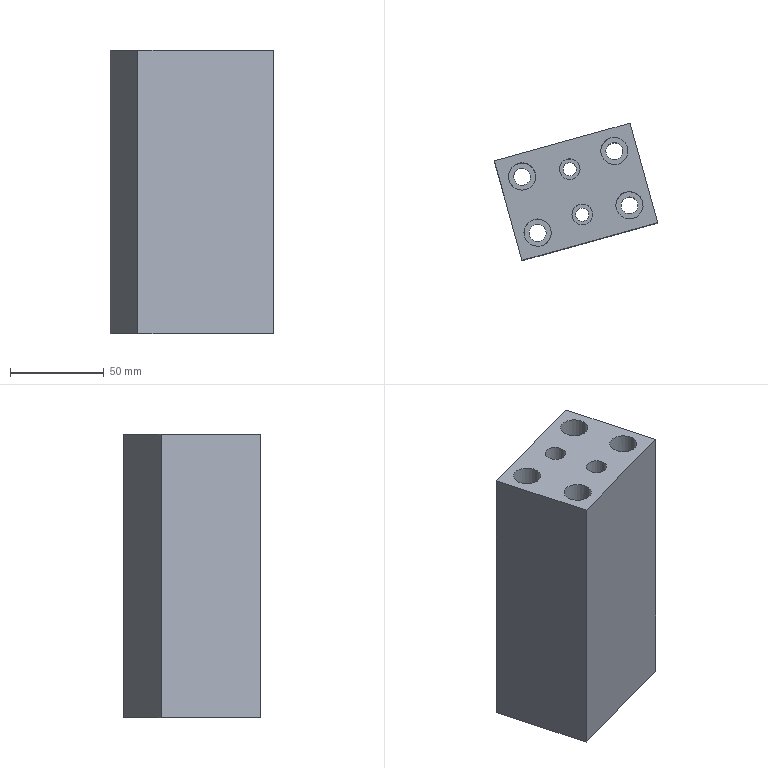Part | NX | features solid 2 | 1 solid | 26 faces | box 86.97 x 73.043 x 151.131 mm | volume 455545 mm3 | plane 13 | cylinder 13 | commonest cylinder face diameters 9.007 x4 14.508 x4 7 x2 11 x2 41 x1
STEP:
#1=CARTESIAN_POINT('',(1601.628,0.6566,173.999));
#2=VERTEX_POINT('',#1);
#3=CARTESIAN_POINT('',(1602.832,-3.683,173.999));
#4=DIRECTION('',(0.,0.,-1.));
#5=DIRECTION('',(-0.2672,0.9636,0.));
#6=AXIS2_PLACEMENT_3D('',#3,#4,#5);
#7=CIRCLE('',#6,4.503);
#8=EDGE_CURVE('',#2,#2,#7,.T.);
#9=ORIENTED_EDGE('',*,*,#8,.T.);
#10=EDGE_LOOP('',(#9));
#11=FACE_BOUND('',#10,.T.);
#12=CARTESIAN_POINT('',(1600.893,3.307,173.999));
#13=VERTEX_POINT('',#12);
#14=CARTESIAN_POINT('',(1602.832,-3.683,173.999));
#15=DIRECTION('',(0.,0.,1.));
#16=DIRECTION('',(-0.2672,0.9636,0.));
#17=AXIS2_PLACEMENT_3D('',#14,#15,#16);
#18=CIRCLE('',#17,7.254);
#19=EDGE_CURVE('',#13,#13,#18,.F.);
#20=ORIENTED_EDGE('',*,*,#19,.F.);
#21=EDGE_LOOP('',(#20));
#22=FACE_BOUND('',#21,.T.);
#23=CARTESIAN_POINT('',(1602.832,-3.683,173.999));
#24=DIRECTION('',(0.,0.,-1.));
#25=DIRECTION('',(-0.2672,0.9636,0.));
#26=AXIS2_PLACEMENT_3D('',#23,#24,#25);
#27=PLANE('',#26);
#28=ADVANCED_FACE('',(#11,#22),#27,.F.);
#29=ORIENTED_EDGE('',*,*,#8,.F.);
#30=EDGE_LOOP('',(#29));
#31=FACE_BOUND('',#30,.T.);
#32=CARTESIAN_POINT('',(1601.628,0.6566,94.999));
#33=VERTEX_POINT('',#32);
#34=CARTESIAN_POINT('',(1602.832,-3.683,94.999));
#35=DIRECTION('',(0.,0.,-1.));
#36=DIRECTION('',(-0.2672,0.9636,0.));
#37=AXIS2_PLACEMENT_3D('',#34,#35,#36);
#38=CIRCLE('',#37,4.503);
#39=EDGE_CURVE('',#33,#33,#38,.T.);
#40=ORIENTED_EDGE('',*,*,#39,.T.);
#41=EDGE_LOOP('',(#40));
#42=FACE_BOUND('',#41,.T.);
#43=CARTESIAN_POINT('',(1602.832,-3.683,187.999));
#44=DIRECTION('',(0.,0.,-1.));
#45=DIRECTION('',(-0.2672,0.9636,0.));
#46=AXIS2_PLACEMENT_3D('',#43,#44,#45);
#47=CYLINDRICAL_SURFACE('',#46,4.503);
#48=ADVANCED_FACE('',(#31,#42),#47,.F.);
#49=ORIENTED_EDGE('',*,*,#19,.T.);
#50=EDGE_LOOP('',(#49));
#51=FACE_BOUND('',#50,.T.);
#52=CARTESIAN_POINT('',(1595.578,-3.683,246.13));
#53=VERTEX_POINT('',#52);
#54=CARTESIAN_POINT('',(1602.832,-3.683,246.13));
#55=DIRECTION('',(0.,0.,-1.));
#56=DIRECTION('',(-1.,0.,0.));
#57=AXIS2_PLACEMENT_3D('',#54,#55,#56);
#58=CIRCLE('',#57,7.254);
#59=EDGE_CURVE('',#53,#53,#58,.F.);
#60=ORIENTED_EDGE('',*,*,#59,.T.);
#61=EDGE_LOOP('',(#60));
#62=FACE_BOUND('',#61,.T.);
#63=CARTESIAN_POINT('',(1602.832,-3.683,184.999));
#64=DIRECTION('',(0.,0.,-1.));
#65=DIRECTION('',(-0.2672,0.9636,0.));
#66=AXIS2_PLACEMENT_3D('',#63,#64,#65);
#67=CYLINDRICAL_SURFACE('',#66,7.254);
#68=ADVANCED_FACE('',(#51,#62),#67,.F.);
#69=CARTESIAN_POINT('',(1616.422,30.113,159.999));
#70=VERTEX_POINT('',#69);
#71=CARTESIAN_POINT('',(1619.922,30.113,159.999));
#72=DIRECTION('',(0.,0.,-1.));
#73=DIRECTION('',(-1.,0.,0.));
#74=AXIS2_PLACEMENT_3D('',#71,#72,#73);
#75=CIRCLE('',#74,3.5);
#76=EDGE_CURVE('',#70,#70,#75,.F.);
#77=ORIENTED_EDGE('',*,*,#76,.F.);
#78=EDGE_LOOP('',(#77));
#79=FACE_BOUND('',#78,.T.);
#80=CARTESIAN_POINT('',(1616.422,30.113,178.999));
#81=VERTEX_POINT('',#80);
#82=CARTESIAN_POINT('',(1619.922,30.113,178.999));
#83=DIRECTION('',(0.,0.,-1.));
#84=DIRECTION('',(-1.,0.,0.));
#85=AXIS2_PLACEMENT_3D('',#82,#83,#84);
#86=CIRCLE('',#85,3.5);
#87=EDGE_CURVE('',#81,#81,#86,.T.);
#88=ORIENTED_EDGE('',*,*,#87,.F.);
#89=EDGE_LOOP('',(#88));
#90=FACE_BOUND('',#89,.T.);
#91=CARTESIAN_POINT('',(1619.922,30.113,201.999));
#92=DIRECTION('',(0.,0.,-1.));
#93=DIRECTION('',(0.2672,-0.9636,0.));
#94=AXIS2_PLACEMENT_3D('',#91,#92,#93);
#95=CYLINDRICAL_SURFACE('',#94,3.5);
#96=ADVANCED_FACE('',(#79,#90),#95,.F.);
#97=CARTESIAN_POINT('',(1623.102,6.022,159.999));
#98=VERTEX_POINT('',#97);
#99=CARTESIAN_POINT('',(1626.602,6.022,159.999));
#100=DIRECTION('',(0.,0.,-1.));
#101=DIRECTION('',(-1.,0.,0.));
#102=AXIS2_PLACEMENT_3D('',#99,#100,#101);
#103=CIRCLE('',#102,3.5);
#104=EDGE_CURVE('',#98,#98,#103,.F.);
#105=ORIENTED_EDGE('',*,*,#104,.F.);
#106=EDGE_LOOP('',(#105));
#107=FACE_BOUND('',#106,.T.);
#108=CARTESIAN_POINT('',(1623.102,6.022,178.999));
#109=VERTEX_POINT('',#108);
#110=CARTESIAN_POINT('',(1626.602,6.022,178.999));
#111=DIRECTION('',(0.,0.,-1.));
#112=DIRECTION('',(-1.,0.,0.));
#113=AXIS2_PLACEMENT_3D('',#110,#111,#112);
#114=CIRCLE('',#113,3.5);
#115=EDGE_CURVE('',#109,#109,#114,.T.);
#116=ORIENTED_EDGE('',*,*,#115,.F.);
#117=EDGE_LOOP('',(#116));
#118=FACE_BOUND('',#117,.T.);
#119=CARTESIAN_POINT('',(1626.602,6.022,201.999));
#120=DIRECTION('',(0.,0.,-1.));
#121=DIRECTION('',(0.2672,-0.9636,0.));
#122=AXIS2_PLACEMENT_3D('',#119,#120,#121);
#123=CYLINDRICAL_SURFACE('',#122,3.5);
#124=ADVANCED_FACE('',(#107,#118),#123,.F.);
#125=ORIENTED_EDGE('',*,*,#115,.T.);
#126=EDGE_LOOP('',(#125));
#127=FACE_BOUND('',#126,.T.);
#128=CARTESIAN_POINT('',(1621.102,6.022,178.999));
#129=VERTEX_POINT('',#128);
#130=CARTESIAN_POINT('',(1626.602,6.022,178.999));
#131=DIRECTION('',(0.,0.,-1.));
#132=DIRECTION('',(-1.,0.,0.));
#133=AXIS2_PLACEMENT_3D('',#130,#131,#132);
#134=CIRCLE('',#133,5.5);
#135=EDGE_CURVE('',#129,#129,#134,.T.);
#136=ORIENTED_EDGE('',*,*,#135,.F.);
#137=EDGE_LOOP('',(#136));
#138=FACE_BOUND('',#137,.T.);
#139=CARTESIAN_POINT('',(1626.602,6.022,178.999));
#140=DIRECTION('',(0.,0.,-1.));
#141=DIRECTION('',(-0.2672,0.9636,0.));
#142=AXIS2_PLACEMENT_3D('',#139,#140,#141);
#143=PLANE('',#142);
#144=ADVANCED_FACE('',(#127,#138),#143,.F.);
#145=ORIENTED_EDGE('',*,*,#87,.T.);
#146=EDGE_LOOP('',(#145));
#147=FACE_BOUND('',#146,.T.);
#148=CARTESIAN_POINT('',(1614.422,30.113,178.999));
#149=VERTEX_POINT('',#148);
#150=CARTESIAN_POINT('',(1619.922,30.113,178.999));
#151=DIRECTION('',(0.,0.,-1.));
#152=DIRECTION('',(-1.,0.,0.));
#153=AXIS2_PLACEMENT_3D('',#150,#151,#152);
#154=CIRCLE('',#153,5.5);
#155=EDGE_CURVE('',#149,#149,#154,.T.);
#156=ORIENTED_EDGE('',*,*,#155,.F.);
#157=EDGE_LOOP('',(#156));
#158=FACE_BOUND('',#157,.T.);
#159=CARTESIAN_POINT('',(1619.922,30.113,178.999));
#160=DIRECTION('',(0.,0.,-1.));
#161=DIRECTION('',(-0.2672,0.9636,0.));
#162=AXIS2_PLACEMENT_3D('',#159,#160,#161);
#163=PLANE('',#162);
#164=ADVANCED_FACE('',(#147,#158),#163,.F.);
#165=ORIENTED_EDGE('',*,*,#104,.T.);
#166=EDGE_LOOP('',(#165));
#167=FACE_BOUND('',#166,.T.);
#168=CARTESIAN_POINT('',(1617.784,37.822,159.999));
#169=VERTEX_POINT('',#168);
#170=CARTESIAN_POINT('',(1623.262,18.068,159.999));
#171=DIRECTION('',(0.,0.,-1.));
#172=DIRECTION('',(-0.2672,0.9636,0.));
#173=AXIS2_PLACEMENT_3D('',#170,#171,#172);
#174=CIRCLE('',#173,20.5);
#175=EDGE_CURVE('',#169,#169,#174,.T.);
#176=ORIENTED_EDGE('',*,*,#175,.T.);
#177=EDGE_LOOP('',(#176));
#178=FACE_BOUND('',#177,.T.);
#179=ORIENTED_EDGE('',*,*,#76,.T.);
#180=EDGE_LOOP('',(#179));
#181=FACE_BOUND('',#180,.T.);
#182=CARTESIAN_POINT('',(1623.262,18.068,159.999));
#183=DIRECTION('',(0.,0.,-1.));
#184=DIRECTION('',(-0.2672,0.9636,0.));
#185=AXIS2_PLACEMENT_3D('',#182,#183,#184);
#186=PLANE('',#185);
#187=ADVANCED_FACE('',(#167,#178,#181),#186,.T.);
#188=CARTESIAN_POINT('',(1652.913,6.57,173.999));
#189=VERTEX_POINT('',#188);
#190=CARTESIAN_POINT('',(1651.71,10.91,173.999));
#191=DIRECTION('',(0.,0.,1.));
#192=DIRECTION('',(0.2672,-0.9636,0.));
#193=AXIS2_PLACEMENT_3D('',#190,#191,#192);
#194=CIRCLE('',#193,4.503);
#195=EDGE_CURVE('',#189,#189,#194,.F.);
#196=ORIENTED_EDGE('',*,*,#195,.T.);
#197=EDGE_LOOP('',(#196));
#198=FACE_BOUND('',#197,.T.);
#199=CARTESIAN_POINT('',(1653.648,3.92,173.999));
#200=VERTEX_POINT('',#199);
#201=CARTESIAN_POINT('',(1651.71,10.91,173.999));
#202=DIRECTION('',(0.,0.,-1.));
#203=DIRECTION('',(0.2672,-0.9636,0.));
#204=AXIS2_PLACEMENT_3D('',#201,#202,#203);
#205=CIRCLE('',#204,7.254);
#206=EDGE_CURVE('',#200,#200,#205,.T.);
#207=ORIENTED_EDGE('',*,*,#206,.F.);
#208=EDGE_LOOP('',(#207));
#209=FACE_BOUND('',#208,.T.);
#210=CARTESIAN_POINT('',(1651.71,10.91,173.999));
#211=DIRECTION('',(0.,0.,-1.));
#212=DIRECTION('',(0.2672,-0.9636,0.));
#213=AXIS2_PLACEMENT_3D('',#210,#211,#212);
#214=PLANE('',#213);
#215=ADVANCED_FACE('',(#198,#209),#214,.F.);
#216=CARTESIAN_POINT('',(1644.896,35.479,173.999));
#217=VERTEX_POINT('',#216);
#218=CARTESIAN_POINT('',(1643.692,39.819,173.999));
#219=DIRECTION('',(0.,0.,1.));
#220=DIRECTION('',(0.2672,-0.9636,0.));
#221=AXIS2_PLACEMENT_3D('',#218,#219,#220);
#222=CIRCLE('',#221,4.503);
#223=EDGE_CURVE('',#217,#217,#222,.F.);
#224=ORIENTED_EDGE('',*,*,#223,.T.);
#225=EDGE_LOOP('',(#224));
#226=FACE_BOUND('',#225,.T.);
#227=CARTESIAN_POINT('',(1645.631,32.828,173.999));
#228=VERTEX_POINT('',#227);
#229=CARTESIAN_POINT('',(1643.692,39.819,173.999));
#230=DIRECTION('',(0.,0.,-1.));
#231=DIRECTION('',(0.2672,-0.9636,0.));
#232=AXIS2_PLACEMENT_3D('',#229,#230,#231);
#233=CIRCLE('',#232,7.254);
#234=EDGE_CURVE('',#228,#228,#233,.T.);
#235=ORIENTED_EDGE('',*,*,#234,.F.);
#236=EDGE_LOOP('',(#235));
#237=FACE_BOUND('',#236,.T.);
#238=CARTESIAN_POINT('',(1643.692,39.819,173.999));
#239=DIRECTION('',(0.,0.,-1.));
#240=DIRECTION('',(0.2672,-0.9636,0.));
#241=AXIS2_PLACEMENT_3D('',#238,#239,#240);
#242=PLANE('',#241);
#243=ADVANCED_FACE('',(#226,#237),#242,.F.);
#244=CARTESIAN_POINT('',(1595.751,21.85,173.999));
#245=VERTEX_POINT('',#244);
#246=CARTESIAN_POINT('',(1594.547,26.189,173.999));
#247=DIRECTION('',(0.,0.,1.));
#248=DIRECTION('',(0.2672,-0.9636,0.));
#249=AXIS2_PLACEMENT_3D('',#246,#247,#248);
#250=CIRCLE('',#249,4.503);
#251=EDGE_CURVE('',#245,#245,#250,.F.);
#252=ORIENTED_EDGE('',*,*,#251,.T.);
#253=EDGE_LOOP('',(#252));
#254=FACE_BOUND('',#253,.T.);
#255=CARTESIAN_POINT('',(1596.486,19.199,173.999));
#256=VERTEX_POINT('',#255);
#257=CARTESIAN_POINT('',(1594.547,26.189,173.999));
#258=DIRECTION('',(0.,0.,-1.));
#259=DIRECTION('',(0.2672,-0.9636,0.));
#260=AXIS2_PLACEMENT_3D('',#257,#258,#259);
#261=CIRCLE('',#260,7.254);
#262=EDGE_CURVE('',#256,#256,#261,.T.);
#263=ORIENTED_EDGE('',*,*,#262,.F.);
#264=EDGE_LOOP('',(#263));
#265=FACE_BOUND('',#264,.T.);
#266=CARTESIAN_POINT('',(1594.547,26.189,173.999));
#267=DIRECTION('',(0.,0.,-1.));
#268=DIRECTION('',(0.2672,-0.9636,0.));
#269=AXIS2_PLACEMENT_3D('',#266,#267,#268);
#270=PLANE('',#269);
#271=ADVANCED_FACE('',(#254,#265),#270,.F.);
#272=ORIENTED_EDGE('',*,*,#206,.T.);
#273=EDGE_LOOP('',(#272));
#274=FACE_BOUND('',#273,.T.);
#275=CARTESIAN_POINT('',(1644.456,10.91,246.13));
#276=VERTEX_POINT('',#275);
#277=CARTESIAN_POINT('',(1651.71,10.91,246.13));
#278=DIRECTION('',(0.,0.,-1.));
#279=DIRECTION('',(-1.,0.,0.));
#280=AXIS2_PLACEMENT_3D('',#277,#278,#279);
#281=CIRCLE('',#280,7.254);
#282=EDGE_CURVE('',#276,#276,#281,.T.);
#283=ORIENTED_EDGE('',*,*,#282,.F.);
#284=EDGE_LOOP('',(#283));
#285=FACE_BOUND('',#284,.T.);
#286=CARTESIAN_POINT('',(1651.71,10.91,184.999));
#287=DIRECTION('',(0.,0.,-1.));
#288=DIRECTION('',(0.2672,-0.9636,0.));
#289=AXIS2_PLACEMENT_3D('',#286,#287,#288);
#290=CYLINDRICAL_SURFACE('',#289,7.254);
#291=ADVANCED_FACE('',(#274,#285),#290,.F.);
#292=ORIENTED_EDGE('',*,*,#262,.T.);
#293=EDGE_LOOP('',(#292));
#294=FACE_BOUND('',#293,.T.);
#295=CARTESIAN_POINT('',(1587.293,26.189,246.13));
#296=VERTEX_POINT('',#295);
#297=CARTESIAN_POINT('',(1594.547,26.189,246.13));
#298=DIRECTION('',(0.,0.,-1.));
#299=DIRECTION('',(-1.,0.,0.));
#300=AXIS2_PLACEMENT_3D('',#297,#298,#299);
#301=CIRCLE('',#300,7.254);
#302=EDGE_CURVE('',#296,#296,#301,.T.);
#303=ORIENTED_EDGE('',*,*,#302,.F.);
#304=EDGE_LOOP('',(#303));
#305=FACE_BOUND('',#304,.T.);
#306=CARTESIAN_POINT('',(1594.547,26.189,184.999));
#307=DIRECTION('',(0.,0.,-1.));
#308=DIRECTION('',(0.2672,-0.9636,0.));
#309=AXIS2_PLACEMENT_3D('',#306,#307,#308);
#310=CYLINDRICAL_SURFACE('',#309,7.254);
#311=ADVANCED_FACE('',(#294,#305),#310,.F.);
#312=ORIENTED_EDGE('',*,*,#234,.T.);
#313=EDGE_LOOP('',(#312));
#314=FACE_BOUND('',#313,.T.);
#315=CARTESIAN_POINT('',(1636.438,39.819,246.13));
#316=VERTEX_POINT('',#315);
#317=CARTESIAN_POINT('',(1643.692,39.819,246.13));
#318=DIRECTION('',(0.,0.,-1.));
#319=DIRECTION('',(-1.,0.,0.));
#320=AXIS2_PLACEMENT_3D('',#317,#318,#319);
#321=CIRCLE('',#320,7.254);
#322=EDGE_CURVE('',#316,#316,#321,.T.);
#323=ORIENTED_EDGE('',*,*,#322,.F.);
#324=EDGE_LOOP('',(#323));
#325=FACE_BOUND('',#324,.T.);
#326=CARTESIAN_POINT('',(1643.692,39.819,184.999));
#327=DIRECTION('',(0.,0.,-1.));
#328=DIRECTION('',(0.2672,-0.9636,0.));
#329=AXIS2_PLACEMENT_3D('',#326,#327,#328);
#330=CYLINDRICAL_SURFACE('',#329,7.254);
#331=ADVANCED_FACE('',(#314,#325),#330,.F.);
#332=CARTESIAN_POINT('',(1621.102,6.022,246.13));
#333=VERTEX_POINT('',#332);
#334=CARTESIAN_POINT('',(1626.602,6.022,246.13));
#335=DIRECTION('',(0.,0.,-1.));
#336=DIRECTION('',(-1.,0.,0.));
#337=AXIS2_PLACEMENT_3D('',#334,#335,#336);
#338=CIRCLE('',#337,5.5);
#339=EDGE_CURVE('',#333,#333,#338,.F.);
#340=ORIENTED_EDGE('',*,*,#339,.T.);
#341=EDGE_LOOP('',(#340));
#342=FACE_BOUND('',#341,.T.);
#343=ORIENTED_EDGE('',*,*,#135,.T.);
#344=EDGE_LOOP('',(#343));
#345=FACE_BOUND('',#344,.T.);
#346=CARTESIAN_POINT('',(1626.602,6.022,201.999));
#347=DIRECTION('',(0.,0.,-1.));
#348=DIRECTION('',(0.2672,-0.9636,0.));
#349=AXIS2_PLACEMENT_3D('',#346,#347,#348);
#350=CYLINDRICAL_SURFACE('',#349,5.5);
#351=ADVANCED_FACE('',(#342,#345),#350,.F.);
#352=CARTESIAN_POINT('',(1614.422,30.113,246.13));
#353=VERTEX_POINT('',#352);
#354=CARTESIAN_POINT('',(1619.922,30.113,246.13));
#355=DIRECTION('',(0.,0.,-1.));
#356=DIRECTION('',(-1.,0.,0.));
#357=AXIS2_PLACEMENT_3D('',#354,#355,#356);
#358=CIRCLE('',#357,5.5);
#359=EDGE_CURVE('',#353,#353,#358,.F.);
#360=ORIENTED_EDGE('',*,*,#359,.T.);
#361=EDGE_LOOP('',(#360));
#362=FACE_BOUND('',#361,.T.);
#363=ORIENTED_EDGE('',*,*,#155,.T.);
#364=EDGE_LOOP('',(#363));
#365=FACE_BOUND('',#364,.T.);
#366=CARTESIAN_POINT('',(1619.922,30.113,201.999));
#367=DIRECTION('',(0.,0.,-1.));
#368=DIRECTION('',(0.2672,-0.9636,0.));
#369=AXIS2_PLACEMENT_3D('',#366,#367,#368);
#370=CYLINDRICAL_SURFACE('',#369,5.5);
#371=ADVANCED_FACE('',(#362,#365),#370,.F.);
#372=CARTESIAN_POINT('',(1617.784,37.822,94.999));
#373=VERTEX_POINT('',#372);
#374=CARTESIAN_POINT('',(1623.262,18.068,94.999));
#375=DIRECTION('',(0.,0.,-1.));
#376=DIRECTION('',(-0.2672,0.9636,0.));
#377=AXIS2_PLACEMENT_3D('',#374,#375,#376);
#378=CIRCLE('',#377,20.5);
#379=EDGE_CURVE('',#373,#373,#378,.F.);
#380=ORIENTED_EDGE('',*,*,#379,.F.);
#381=EDGE_LOOP('',(#380));
#382=FACE_BOUND('',#381,.T.);
#383=ORIENTED_EDGE('',*,*,#175,.F.);
#384=EDGE_LOOP('',(#383));
#385=FACE_BOUND('',#384,.T.);
#386=CARTESIAN_POINT('',(1623.262,18.068,1037.539));
#387=DIRECTION('',(0.,0.,-1.));
#388=DIRECTION('',(-0.9681,0.2504,0.));
#389=AXIS2_PLACEMENT_3D('',#386,#387,#388);
#390=CYLINDRICAL_SURFACE('',#389,20.5);
#391=ADVANCED_FACE('',(#382,#385),#390,.F.);
#392=ORIENTED_EDGE('',*,*,#195,.F.);
#393=EDGE_LOOP('',(#392));
#394=FACE_BOUND('',#393,.T.);
#395=CARTESIAN_POINT('',(1650.506,15.249,94.999));
#396=VERTEX_POINT('',#395);
#397=CARTESIAN_POINT('',(1651.71,10.91,94.999));
#398=DIRECTION('',(0.,0.,-1.));
#399=DIRECTION('',(-0.2672,0.9636,0.));
#400=AXIS2_PLACEMENT_3D('',#397,#398,#399);
#401=CIRCLE('',#400,4.503);
#402=EDGE_CURVE('',#396,#396,#401,.F.);
#403=ORIENTED_EDGE('',*,*,#402,.F.);
#404=EDGE_LOOP('',(#403));
#405=FACE_BOUND('',#404,.T.);
#406=CARTESIAN_POINT('',(1651.71,10.91,187.999));
#407=DIRECTION('',(0.,0.,-1.));
#408=DIRECTION('',(0.2672,-0.9636,0.));
#409=AXIS2_PLACEMENT_3D('',#406,#407,#408);
#410=CYLINDRICAL_SURFACE('',#409,4.503);
#411=ADVANCED_FACE('',(#394,#405),#410,.F.);
#412=ORIENTED_EDGE('',*,*,#223,.F.);
#413=EDGE_LOOP('',(#412));
#414=FACE_BOUND('',#413,.T.);
#415=CARTESIAN_POINT('',(1642.489,44.158,94.999));
#416=VERTEX_POINT('',#415);
#417=CARTESIAN_POINT('',(1643.692,39.819,94.999));
#418=DIRECTION('',(0.,0.,-1.));
#419=DIRECTION('',(-0.2672,0.9636,0.));
#420=AXIS2_PLACEMENT_3D('',#417,#418,#419);
#421=CIRCLE('',#420,4.503);
#422=EDGE_CURVE('',#416,#416,#421,.T.);
#423=ORIENTED_EDGE('',*,*,#422,.T.);
#424=EDGE_LOOP('',(#423));
#425=FACE_BOUND('',#424,.T.);
#426=CARTESIAN_POINT('',(1643.692,39.819,187.999));
#427=DIRECTION('',(0.,0.,-1.));
#428=DIRECTION('',(0.2672,-0.9636,0.));
#429=AXIS2_PLACEMENT_3D('',#426,#427,#428);
#430=CYLINDRICAL_SURFACE('',#429,4.503);
#431=ADVANCED_FACE('',(#414,#425),#430,.F.);
#432=ORIENTED_EDGE('',*,*,#251,.F.);
#433=EDGE_LOOP('',(#432));
#434=FACE_BOUND('',#433,.T.);
#435=CARTESIAN_POINT('',(1593.344,30.529,94.999));
#436=VERTEX_POINT('',#435);
#437=CARTESIAN_POINT('',(1594.547,26.189,94.999));
#438=DIRECTION('',(0.,0.,-1.));
#439=DIRECTION('',(-0.2672,0.9636,0.));
#440=AXIS2_PLACEMENT_3D('',#437,#438,#439);
#441=CIRCLE('',#440,4.503);
#442=EDGE_CURVE('',#436,#436,#441,.T.);
#443=ORIENTED_EDGE('',*,*,#442,.T.);
#444=EDGE_LOOP('',(#443));
#445=FACE_BOUND('',#444,.T.);
#446=CARTESIAN_POINT('',(1594.547,26.189,187.999));
#447=DIRECTION('',(0.,0.,-1.));
#448=DIRECTION('',(0.2672,-0.9636,0.));
#449=AXIS2_PLACEMENT_3D('',#446,#447,#448);
#450=CYLINDRICAL_SURFACE('',#449,4.503);
#451=ADVANCED_FACE('',(#434,#445),#450,.F.);
#452=CARTESIAN_POINT('',(1666.747,1.589,246.13));
#453=VERTEX_POINT('',#452);
#454=CARTESIAN_POINT('',(1666.747,1.589,94.999));
#455=VERTEX_POINT('',#454);
#456=CARTESIAN_POINT('',(1666.747,1.589,184.999));
#457=DIRECTION('',(0.,0.,1.));
#458=VECTOR('',#457,1000.);
#459=LINE('',#456,#458);
#460=EDGE_CURVE('',#453,#455,#459,.F.);
#461=ORIENTED_EDGE('',*,*,#460,.T.);
#462=CARTESIAN_POINT('',(1652.049,54.589,94.999));
#463=VERTEX_POINT('',#462);
#464=CARTESIAN_POINT('',(1659.398,28.089,94.999));
#465=DIRECTION('',(-0.2672,0.9636,0.));
#466=VECTOR('',#465,1000.);
#467=LINE('',#464,#466);
#468=EDGE_CURVE('',#455,#463,#467,.T.);
#469=ORIENTED_EDGE('',*,*,#468,.T.);
#470=CARTESIAN_POINT('',(1652.049,54.589,246.13));
#471=VERTEX_POINT('',#470);
#472=CARTESIAN_POINT('',(1652.049,54.589,184.999));
#473=DIRECTION('',(0.,0.,-1.));
#474=VECTOR('',#473,1000.);
#475=LINE('',#472,#474);
#476=EDGE_CURVE('',#463,#471,#475,.F.);
#477=ORIENTED_EDGE('',*,*,#476,.T.);
#478=CARTESIAN_POINT('',(1659.398,28.089,246.13));
#479=DIRECTION('',(-0.2672,0.9636,0.));
#480=VECTOR('',#479,1000.);
#481=LINE('',#478,#480);
#482=EDGE_CURVE('',#471,#453,#481,.F.);
#483=ORIENTED_EDGE('',*,*,#482,.T.);
#484=EDGE_LOOP('',(#461,#469,#477,#483));
#485=FACE_BOUND('',#484,.T.);
#486=CARTESIAN_POINT('',(1659.398,28.089,184.999));
#487=DIRECTION('',(0.9636,0.2672,0.));
#488=DIRECTION('',(0.,0.,-1.));
#489=AXIS2_PLACEMENT_3D('',#486,#487,#488);
#490=PLANE('',#489);
#491=ADVANCED_FACE('',(#485),#490,.T.);
#492=ORIENTED_EDGE('',*,*,#476,.F.);
#493=CARTESIAN_POINT('',(1579.777,34.546,94.999));
#494=VERTEX_POINT('',#493);
#495=CARTESIAN_POINT('',(1615.913,44.568,94.999));
#496=DIRECTION('',(-0.9636,-0.2672,0.));
#497=VECTOR('',#496,1000.);
#498=LINE('',#495,#497);
#499=EDGE_CURVE('',#463,#494,#498,.T.);
#500=ORIENTED_EDGE('',*,*,#499,.T.);
#501=CARTESIAN_POINT('',(1579.777,34.546,246.13));
#502=VERTEX_POINT('',#501);
#503=CARTESIAN_POINT('',(1579.777,34.546,184.999));
#504=DIRECTION('',(0.,0.,-1.));
#505=VECTOR('',#504,1000.);
#506=LINE('',#503,#505);
#507=EDGE_CURVE('',#494,#502,#506,.F.);
#508=ORIENTED_EDGE('',*,*,#507,.T.);
#509=CARTESIAN_POINT('',(1615.913,44.568,246.13));
#510=DIRECTION('',(-0.9636,-0.2672,0.));
#511=VECTOR('',#510,1000.);
#512=LINE('',#509,#511);
#513=EDGE_CURVE('',#502,#471,#512,.F.);
#514=ORIENTED_EDGE('',*,*,#513,.T.);
#515=EDGE_LOOP('',(#492,#500,#508,#514));
#516=FACE_BOUND('',#515,.T.);
#517=CARTESIAN_POINT('',(1615.913,44.568,184.999));
#518=DIRECTION('',(-0.2672,0.9636,0.));
#519=DIRECTION('',(0.,0.,-1.));
#520=AXIS2_PLACEMENT_3D('',#517,#518,#519);
#521=PLANE('',#520);
#522=ADVANCED_FACE('',(#516),#521,.T.);
#523=CARTESIAN_POINT('',(1594.475,-18.454,94.999));
#524=VERTEX_POINT('',#523);
#525=CARTESIAN_POINT('',(1594.475,-18.454,246.13));
#526=VERTEX_POINT('',#525);
#527=CARTESIAN_POINT('',(1594.475,-18.454,184.999));
#528=DIRECTION('',(0.,0.,-1.));
#529=VECTOR('',#528,1000.);
#530=LINE('',#527,#529);
#531=EDGE_CURVE('',#524,#526,#530,.F.);
#532=ORIENTED_EDGE('',*,*,#531,.T.);
#533=CARTESIAN_POINT('',(1587.126,8.046,246.13));
#534=DIRECTION('',(0.2672,-0.9636,0.));
#535=VECTOR('',#534,1000.);
#536=LINE('',#533,#535);
#537=EDGE_CURVE('',#526,#502,#536,.F.);
#538=ORIENTED_EDGE('',*,*,#537,.T.);
#539=ORIENTED_EDGE('',*,*,#507,.F.);
#540=CARTESIAN_POINT('',(1587.126,8.046,94.999));
#541=DIRECTION('',(0.2672,-0.9636,0.));
#542=VECTOR('',#541,1000.);
#543=LINE('',#540,#542);
#544=EDGE_CURVE('',#494,#524,#543,.T.);
#545=ORIENTED_EDGE('',*,*,#544,.T.);
#546=EDGE_LOOP('',(#532,#538,#539,#545));
#547=FACE_BOUND('',#546,.T.);
#548=CARTESIAN_POINT('',(1587.126,8.046,184.999));
#549=DIRECTION('',(-0.9636,-0.2672,0.));
#550=DIRECTION('',(0.,0.,1.));
#551=AXIS2_PLACEMENT_3D('',#548,#549,#550);
#552=PLANE('',#551);
#553=ADVANCED_FACE('',(#547),#552,.T.);
#554=CARTESIAN_POINT('',(1630.611,-8.432,246.13));
#555=DIRECTION('',(-0.9636,-0.2672,0.));
#556=VECTOR('',#555,1000.);
#557=LINE('',#554,#556);
#558=EDGE_CURVE('',#526,#453,#557,.F.);
#559=ORIENTED_EDGE('',*,*,#558,.F.);
#560=ORIENTED_EDGE('',*,*,#531,.F.);
#561=CARTESIAN_POINT('',(1552.025,-30.226,94.999));
#562=DIRECTION('',(0.9636,0.2672,0.));
#563=VECTOR('',#562,1000.);
#564=LINE('',#561,#563);
#565=EDGE_CURVE('',#455,#524,#564,.F.);
#566=ORIENTED_EDGE('',*,*,#565,.F.);
#567=ORIENTED_EDGE('',*,*,#460,.F.);
#568=EDGE_LOOP('',(#559,#560,#566,#567));
#569=FACE_BOUND('',#568,.T.);
#570=CARTESIAN_POINT('',(1630.611,-8.432,149.065));
#571=DIRECTION('',(-0.2672,0.9636,0.));
#572=DIRECTION('',(0.,0.,1.));
#573=AXIS2_PLACEMENT_3D('',#570,#571,#572);
#574=PLANE('',#573);
#575=ADVANCED_FACE('',(#569),#574,.F.);
#576=ORIENTED_EDGE('',*,*,#39,.F.);
#577=EDGE_LOOP('',(#576));
#578=FACE_BOUND('',#577,.T.);
#579=ORIENTED_EDGE('',*,*,#565,.T.);
#580=ORIENTED_EDGE('',*,*,#544,.F.);
#581=ORIENTED_EDGE('',*,*,#499,.F.);
#582=ORIENTED_EDGE('',*,*,#468,.F.);
#583=EDGE_LOOP('',(#579,#580,#581,#582));
#584=FACE_BOUND('',#583,.T.);
#585=ORIENTED_EDGE('',*,*,#442,.F.);
#586=EDGE_LOOP('',(#585));
#587=FACE_BOUND('',#586,.T.);
#588=ORIENTED_EDGE('',*,*,#422,.F.);
#589=EDGE_LOOP('',(#588));
#590=FACE_BOUND('',#589,.T.);
#591=ORIENTED_EDGE('',*,*,#402,.T.);
#592=EDGE_LOOP('',(#591));
#593=FACE_BOUND('',#592,.T.);
#594=ORIENTED_EDGE('',*,*,#379,.T.);
#595=EDGE_LOOP('',(#594));
#596=FACE_BOUND('',#595,.T.);
#597=CARTESIAN_POINT('',(1553.379,-35.107,94.999));
#598=DIRECTION('',(0.,0.,-1.));
#599=DIRECTION('',(0.2672,-0.9636,0.));
#600=AXIS2_PLACEMENT_3D('',#597,#598,#599);
#601=PLANE('',#600);
#602=ADVANCED_FACE('',(#578,#584,#587,#590,#593,#596),#601,.T.);
#603=ORIENTED_EDGE('',*,*,#59,.F.);
#604=EDGE_LOOP('',(#603));
#605=FACE_BOUND('',#604,.T.);
#606=ORIENTED_EDGE('',*,*,#558,.T.);
#607=ORIENTED_EDGE('',*,*,#482,.F.);
#608=ORIENTED_EDGE('',*,*,#513,.F.);
#609=ORIENTED_EDGE('',*,*,#537,.F.);
#610=EDGE_LOOP('',(#606,#607,#608,#609));
#611=FACE_BOUND('',#610,.T.);
#612=ORIENTED_EDGE('',*,*,#359,.F.);
#613=EDGE_LOOP('',(#612));
#614=FACE_BOUND('',#613,.T.);
#615=ORIENTED_EDGE('',*,*,#339,.F.);
#616=EDGE_LOOP('',(#615));
#617=FACE_BOUND('',#616,.T.);
#618=ORIENTED_EDGE('',*,*,#322,.T.);
#619=EDGE_LOOP('',(#618));
#620=FACE_BOUND('',#619,.T.);
#621=ORIENTED_EDGE('',*,*,#302,.T.);
#622=EDGE_LOOP('',(#621));
#623=FACE_BOUND('',#622,.T.);
#624=ORIENTED_EDGE('',*,*,#282,.T.);
#625=EDGE_LOOP('',(#624));
#626=FACE_BOUND('',#625,.T.);
#627=CARTESIAN_POINT('',(1036.249,1839.888,246.13));
#628=DIRECTION('',(0.,0.,-1.));
#629=DIRECTION('',(-0.2672,0.9636,0.));
#630=AXIS2_PLACEMENT_3D('',#627,#628,#629);
#631=PLANE('',#630);
#632=ADVANCED_FACE('',(#605,#611,#614,#617,#620,#623,#626),#631,.F.);
#633=CLOSED_SHELL('',(#28,#48,#68,#96,#124,#144,#164,#187,#215,#243,#271,#291,#311,#331,#351,#371,#391,#411,#431,#451,#491,#522,#553,#575,#602,#632));
#634=MANIFOLD_SOLID_BREP('',#633);
#635=(LENGTH_UNIT()NAMED_UNIT(*)SI_UNIT(.MILLI.,.METRE.));
#636=UNCERTAINTY_MEASURE_WITH_UNIT(LENGTH_MEASURE(0.00001),#635,'','');
#637=(NAMED_UNIT(*)PLANE_ANGLE_UNIT()SI_UNIT($,.RADIAN.));
#638=(NAMED_UNIT(*)SI_UNIT($,.STERADIAN.)SOLID_ANGLE_UNIT());
#639=(GEOMETRIC_REPRESENTATION_CONTEXT(3)GLOBAL_UNCERTAINTY_ASSIGNED_CONTEXT((#636))GLOBAL_UNIT_ASSIGNED_CONTEXT((#635,#637,#638))REPRESENTATION_CONTEXT('',''));
#640=ADVANCED_BREP_SHAPE_REPRESENTATION('',(#634),#639);